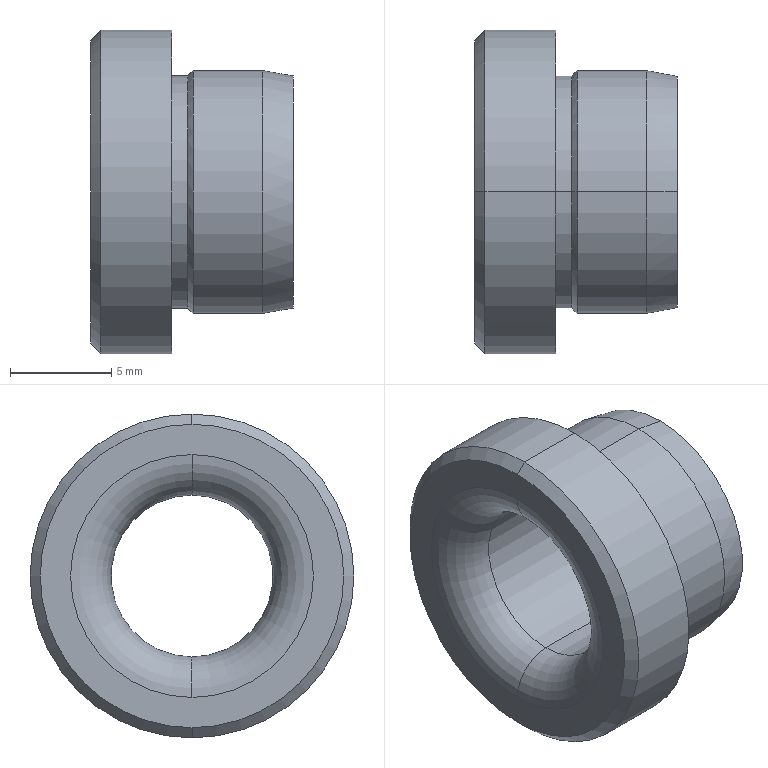Part | NX | features BREP 1 | 1 solid | 23 faces | box 10 x 16 x 16 mm | volume 921.631 mm3 | cylinder 8 | cone 8 | torus 4 | plane 3 | commonest cylinder face diameters 8 x2 11.5 x2 12 x2 16 x2
STEP:
#1=CARTESIAN_POINT('',(0.,0.,6.));
#2=VERTEX_POINT('',#1);
#3=CARTESIAN_POINT('',(0.,0.,-6.));
#4=VERTEX_POINT('',#3);
#5=CARTESIAN_POINT('',(0.,0.,0.));
#6=DIRECTION('',(-1.,0.,0.));
#7=DIRECTION('',(0.,0.,1.));
#8=AXIS2_PLACEMENT_3D('',#5,#6,#7);
#9=CIRCLE('',#8,6.);
#10=EDGE_CURVE('',#2,#4,#9,.T.);
#11=ORIENTED_EDGE('',*,*,#10,.T.);
#12=CARTESIAN_POINT('',(2.,0.,-4.));
#13=VERTEX_POINT('',#12);
#14=CARTESIAN_POINT('',(2.,0.,-6.));
#15=DIRECTION('',(0.,1.,0.));
#16=DIRECTION('',(0.,0.,1.));
#17=AXIS2_PLACEMENT_3D('',#14,#15,#16);
#18=CIRCLE('',#17,2.);
#19=EDGE_CURVE('',#13,#4,#18,.F.);
#20=ORIENTED_EDGE('',*,*,#19,.F.);
#21=CARTESIAN_POINT('',(2.,0.,4.));
#22=VERTEX_POINT('',#21);
#23=CARTESIAN_POINT('',(2.,0.,0.));
#24=DIRECTION('',(-1.,0.,0.));
#25=DIRECTION('',(0.,0.,1.));
#26=AXIS2_PLACEMENT_3D('',#23,#24,#25);
#27=CIRCLE('',#26,4.);
#28=EDGE_CURVE('',#22,#13,#27,.T.);
#29=ORIENTED_EDGE('',*,*,#28,.F.);
#30=CARTESIAN_POINT('',(2.,0.,6.));
#31=DIRECTION('',(0.,-1.,0.));
#32=DIRECTION('',(0.,0.,-1.));
#33=AXIS2_PLACEMENT_3D('',#30,#31,#32);
#34=CIRCLE('',#33,2.);
#35=EDGE_CURVE('',#22,#2,#34,.F.);
#36=ORIENTED_EDGE('',*,*,#35,.T.);
#37=EDGE_LOOP('',(#11,#20,#29,#36));
#38=FACE_BOUND('',#37,.T.);
#39=CARTESIAN_POINT('',(2.,0.,0.));
#40=DIRECTION('',(-1.,0.,0.));
#41=DIRECTION('',(0.,0.,1.));
#42=AXIS2_PLACEMENT_3D('',#39,#40,#41);
#43=TOROIDAL_SURFACE('',#42,6.,2.);
#44=ADVANCED_FACE('',(#38),#43,.T.);
#45=CARTESIAN_POINT('',(10.,0.,-4.));
#46=VERTEX_POINT('',#45);
#47=CARTESIAN_POINT('',(10.,0.,4.));
#48=VERTEX_POINT('',#47);
#49=CARTESIAN_POINT('',(10.,0.,0.));
#50=DIRECTION('',(-1.,0.,0.));
#51=DIRECTION('',(0.,0.,1.));
#52=AXIS2_PLACEMENT_3D('',#49,#50,#51);
#53=CIRCLE('',#52,4.);
#54=EDGE_CURVE('',#46,#48,#53,.T.);
#55=ORIENTED_EDGE('',*,*,#54,.F.);
#56=CARTESIAN_POINT('',(10.,0.,-4.));
#57=DIRECTION('',(-1.,0.,0.));
#58=VECTOR('',#57,1000.);
#59=LINE('',#56,#58);
#60=EDGE_CURVE('',#13,#46,#59,.F.);
#61=ORIENTED_EDGE('',*,*,#60,.F.);
#62=CARTESIAN_POINT('',(2.,0.,0.));
#63=DIRECTION('',(-1.,0.,0.));
#64=DIRECTION('',(0.,0.,1.));
#65=AXIS2_PLACEMENT_3D('',#62,#63,#64);
#66=CIRCLE('',#65,4.);
#67=EDGE_CURVE('',#13,#22,#66,.T.);
#68=ORIENTED_EDGE('',*,*,#67,.T.);
#69=CARTESIAN_POINT('',(10.,0.,4.));
#70=DIRECTION('',(-1.,0.,0.));
#71=VECTOR('',#70,1000.);
#72=LINE('',#69,#71);
#73=EDGE_CURVE('',#22,#48,#72,.F.);
#74=ORIENTED_EDGE('',*,*,#73,.T.);
#75=EDGE_LOOP('',(#55,#61,#68,#74));
#76=FACE_BOUND('',#75,.T.);
#77=CARTESIAN_POINT('',(10.,0.,0.));
#78=DIRECTION('',(-1.,0.,0.));
#79=DIRECTION('',(0.,0.,1.));
#80=AXIS2_PLACEMENT_3D('',#77,#78,#79);
#81=CYLINDRICAL_SURFACE('',#80,4.);
#82=ADVANCED_FACE('',(#76),#81,.F.);
#83=CARTESIAN_POINT('',(8.5,0.,6.));
#84=VERTEX_POINT('',#83);
#85=CARTESIAN_POINT('',(8.5,0.,-6.));
#86=VERTEX_POINT('',#85);
#87=CARTESIAN_POINT('',(8.5,0.,0.));
#88=DIRECTION('',(-1.,0.,0.));
#89=DIRECTION('',(0.,0.,1.));
#90=AXIS2_PLACEMENT_3D('',#87,#88,#89);
#91=CIRCLE('',#90,6.);
#92=EDGE_CURVE('',#84,#86,#91,.T.);
#93=ORIENTED_EDGE('',*,*,#92,.T.);
#94=CARTESIAN_POINT('',(5.05,0.,-6.));
#95=VERTEX_POINT('',#94);
#96=CARTESIAN_POINT('',(10.,0.,-6.));
#97=DIRECTION('',(-1.,0.,0.));
#98=VECTOR('',#97,1000.);
#99=LINE('',#96,#98);
#100=EDGE_CURVE('',#95,#86,#99,.F.);
#101=ORIENTED_EDGE('',*,*,#100,.F.);
#102=CARTESIAN_POINT('',(5.05,0.,6.));
#103=VERTEX_POINT('',#102);
#104=CARTESIAN_POINT('',(5.05,0.,0.));
#105=DIRECTION('',(-1.,0.,0.));
#106=DIRECTION('',(0.,0.,-1.));
#107=AXIS2_PLACEMENT_3D('',#104,#105,#106);
#108=CIRCLE('',#107,6.);
#109=EDGE_CURVE('',#103,#95,#108,.T.);
#110=ORIENTED_EDGE('',*,*,#109,.F.);
#111=CARTESIAN_POINT('',(10.,0.,6.));
#112=DIRECTION('',(-1.,0.,0.));
#113=VECTOR('',#112,1000.);
#114=LINE('',#111,#113);
#115=EDGE_CURVE('',#103,#84,#114,.F.);
#116=ORIENTED_EDGE('',*,*,#115,.T.);
#117=EDGE_LOOP('',(#93,#101,#110,#116));
#118=FACE_BOUND('',#117,.T.);
#119=CARTESIAN_POINT('',(10.,0.,0.));
#120=DIRECTION('',(-1.,0.,0.));
#121=DIRECTION('',(0.,0.,1.));
#122=AXIS2_PLACEMENT_3D('',#119,#120,#121);
#123=CYLINDRICAL_SURFACE('',#122,6.);
#124=ADVANCED_FACE('',(#118),#123,.T.);
#125=CARTESIAN_POINT('',(10.,0.,5.736));
#126=VERTEX_POINT('',#125);
#127=CARTESIAN_POINT('',(10.,0.,-5.736));
#128=VERTEX_POINT('',#127);
#129=CARTESIAN_POINT('',(10.,0.,0.));
#130=DIRECTION('',(-1.,0.,0.));
#131=DIRECTION('',(0.,0.,1.));
#132=AXIS2_PLACEMENT_3D('',#129,#130,#131);
#133=CIRCLE('',#132,5.736);
#134=EDGE_CURVE('',#126,#128,#133,.T.);
#135=ORIENTED_EDGE('',*,*,#134,.T.);
#136=CARTESIAN_POINT('',(10.,0.,-5.736));
#137=DIRECTION('',(-0.9848,0.,-0.1736));
#138=VECTOR('',#137,1000.);
#139=LINE('',#136,#138);
#140=EDGE_CURVE('',#86,#128,#139,.F.);
#141=ORIENTED_EDGE('',*,*,#140,.F.);
#142=ORIENTED_EDGE('',*,*,#92,.F.);
#143=CARTESIAN_POINT('',(10.,0.,5.736));
#144=DIRECTION('',(-0.9848,0.,0.1736));
#145=VECTOR('',#144,1000.);
#146=LINE('',#143,#145);
#147=EDGE_CURVE('',#84,#126,#146,.F.);
#148=ORIENTED_EDGE('',*,*,#147,.T.);
#149=EDGE_LOOP('',(#135,#141,#142,#148));
#150=FACE_BOUND('',#149,.T.);
#151=CARTESIAN_POINT('',(10.,0.,0.));
#152=DIRECTION('',(-1.,0.,0.));
#153=DIRECTION('',(0.,0.,1.));
#154=AXIS2_PLACEMENT_3D('',#151,#152,#153);
#155=CONICAL_SURFACE('',#154,5.736,0.1745);
#156=ADVANCED_FACE('',(#150),#155,.T.);
#157=CARTESIAN_POINT('',(4.8,0.,5.75));
#158=VERTEX_POINT('',#157);
#159=CARTESIAN_POINT('',(4.8,0.,-5.75));
#160=VERTEX_POINT('',#159);
#161=CARTESIAN_POINT('',(4.8,0.,0.));
#162=DIRECTION('',(-1.,0.,0.));
#163=DIRECTION('',(0.,0.,1.));
#164=AXIS2_PLACEMENT_3D('',#161,#162,#163);
#165=CIRCLE('',#164,5.75);
#166=EDGE_CURVE('',#158,#160,#165,.T.);
#167=ORIENTED_EDGE('',*,*,#166,.T.);
#168=CARTESIAN_POINT('',(4.,0.,-5.75));
#169=VERTEX_POINT('',#168);
#170=CARTESIAN_POINT('',(50.,0.,-5.75));
#171=DIRECTION('',(-1.,0.,0.));
#172=VECTOR('',#171,1000.);
#173=LINE('',#170,#172);
#174=EDGE_CURVE('',#169,#160,#173,.F.);
#175=ORIENTED_EDGE('',*,*,#174,.F.);
#176=CARTESIAN_POINT('',(4.,0.,5.75));
#177=VERTEX_POINT('',#176);
#178=CARTESIAN_POINT('',(4.,0.,0.));
#179=DIRECTION('',(-1.,0.,0.));
#180=DIRECTION('',(0.,0.,1.));
#181=AXIS2_PLACEMENT_3D('',#178,#179,#180);
#182=CIRCLE('',#181,5.75);
#183=EDGE_CURVE('',#177,#169,#182,.T.);
#184=ORIENTED_EDGE('',*,*,#183,.F.);
#185=CARTESIAN_POINT('',(50.,0.,5.75));
#186=DIRECTION('',(-1.,0.,0.));
#187=VECTOR('',#186,1000.);
#188=LINE('',#185,#187);
#189=EDGE_CURVE('',#177,#158,#188,.F.);
#190=ORIENTED_EDGE('',*,*,#189,.T.);
#191=EDGE_LOOP('',(#167,#175,#184,#190));
#192=FACE_BOUND('',#191,.T.);
#193=CARTESIAN_POINT('',(50.,0.,0.));
#194=DIRECTION('',(-1.,0.,0.));
#195=DIRECTION('',(0.,0.,1.));
#196=AXIS2_PLACEMENT_3D('',#193,#194,#195);
#197=CYLINDRICAL_SURFACE('',#196,5.75);
#198=ADVANCED_FACE('',(#192),#197,.T.);
#199=CARTESIAN_POINT('',(3.645,0.,-6.335));
#200=VERTEX_POINT('',#199);
#201=CARTESIAN_POINT('',(3.645,0.,6.335));
#202=VERTEX_POINT('',#201);
#203=CARTESIAN_POINT('',(3.645,0.,0.));
#204=DIRECTION('',(-1.,0.,0.));
#205=DIRECTION('',(0.,0.,1.));
#206=AXIS2_PLACEMENT_3D('',#203,#204,#205);
#207=CIRCLE('',#206,6.335);
#208=EDGE_CURVE('',#200,#202,#207,.T.);
#209=ORIENTED_EDGE('',*,*,#208,.F.);
#210=CARTESIAN_POINT('',(4.,0.,-6.15));
#211=DIRECTION('',(0.,1.,0.));
#212=DIRECTION('',(0.,0.,1.));
#213=AXIS2_PLACEMENT_3D('',#210,#211,#212);
#214=CIRCLE('',#213,0.4);
#215=EDGE_CURVE('',#169,#200,#214,.F.);
#216=ORIENTED_EDGE('',*,*,#215,.F.);
#217=CARTESIAN_POINT('',(4.,0.,0.));
#218=DIRECTION('',(-1.,0.,0.));
#219=DIRECTION('',(0.,0.,1.));
#220=AXIS2_PLACEMENT_3D('',#217,#218,#219);
#221=CIRCLE('',#220,5.75);
#222=EDGE_CURVE('',#169,#177,#221,.T.);
#223=ORIENTED_EDGE('',*,*,#222,.T.);
#224=CARTESIAN_POINT('',(4.,0.,6.15));
#225=DIRECTION('',(0.,-1.,0.));
#226=DIRECTION('',(0.,0.,-1.));
#227=AXIS2_PLACEMENT_3D('',#224,#225,#226);
#228=CIRCLE('',#227,0.4);
#229=EDGE_CURVE('',#177,#202,#228,.F.);
#230=ORIENTED_EDGE('',*,*,#229,.T.);
#231=EDGE_LOOP('',(#209,#216,#223,#230));
#232=FACE_BOUND('',#231,.T.);
#233=CARTESIAN_POINT('',(4.,0.,0.));
#234=DIRECTION('',(-1.,0.,0.));
#235=DIRECTION('',(0.,0.,1.));
#236=AXIS2_PLACEMENT_3D('',#233,#234,#235);
#237=TOROIDAL_SURFACE('',#236,6.15,0.4);
#238=ADVANCED_FACE('',(#232),#237,.F.);
#239=ORIENTED_EDGE('',*,*,#166,.F.);
#240=CARTESIAN_POINT('',(4.8,0.,5.75));
#241=DIRECTION('',(0.7071,0.,0.7071));
#242=VECTOR('',#241,1000.);
#243=LINE('',#240,#242);
#244=EDGE_CURVE('',#158,#103,#243,.T.);
#245=ORIENTED_EDGE('',*,*,#244,.T.);
#246=ORIENTED_EDGE('',*,*,#109,.T.);
#247=CARTESIAN_POINT('',(4.8,0.,-5.75));
#248=DIRECTION('',(0.7071,0.,-0.7071));
#249=VECTOR('',#248,1000.);
#250=LINE('',#247,#249);
#251=EDGE_CURVE('',#160,#95,#250,.T.);
#252=ORIENTED_EDGE('',*,*,#251,.F.);
#253=EDGE_LOOP('',(#239,#245,#246,#252));
#254=FACE_BOUND('',#253,.T.);
#255=CARTESIAN_POINT('',(4.8,0.,0.));
#256=DIRECTION('',(1.,0.,0.));
#257=DIRECTION('',(0.,0.,-1.));
#258=AXIS2_PLACEMENT_3D('',#255,#256,#257);
#259=CONICAL_SURFACE('',#258,5.75,0.7854);
#260=ADVANCED_FACE('',(#254),#259,.T.);
#261=ORIENTED_EDGE('',*,*,#208,.T.);
#262=CARTESIAN_POINT('',(4.,0.,7.016));
#263=VERTEX_POINT('',#262);
#264=CARTESIAN_POINT('',(4.122,0.,7.25));
#265=DIRECTION('',(0.4617,0.,0.887));
#266=VECTOR('',#265,1000.);
#267=LINE('',#264,#266);
#268=EDGE_CURVE('',#202,#263,#267,.T.);
#269=ORIENTED_EDGE('',*,*,#268,.T.);
#270=CARTESIAN_POINT('',(4.,0.,-7.016));
#271=VERTEX_POINT('',#270);
#272=CARTESIAN_POINT('',(4.,0.,0.));
#273=DIRECTION('',(1.,0.,0.));
#274=DIRECTION('',(0.,0.,1.));
#275=AXIS2_PLACEMENT_3D('',#272,#273,#274);
#276=CIRCLE('',#275,7.016);
#277=EDGE_CURVE('',#263,#271,#276,.T.);
#278=ORIENTED_EDGE('',*,*,#277,.T.);
#279=CARTESIAN_POINT('',(4.122,0.,-7.25));
#280=DIRECTION('',(0.4617,0.,-0.887));
#281=VECTOR('',#280,1000.);
#282=LINE('',#279,#281);
#283=EDGE_CURVE('',#200,#271,#282,.T.);
#284=ORIENTED_EDGE('',*,*,#283,.F.);
#285=EDGE_LOOP('',(#261,#269,#278,#284));
#286=FACE_BOUND('',#285,.T.);
#287=CARTESIAN_POINT('',(4.122,0.,0.));
#288=DIRECTION('',(1.,0.,0.));
#289=DIRECTION('',(0.,0.,-1.));
#290=AXIS2_PLACEMENT_3D('',#287,#288,#289);
#291=CONICAL_SURFACE('',#290,7.25,1.091);
#292=ADVANCED_FACE('',(#286),#291,.F.);
#293=CARTESIAN_POINT('',(4.,0.,8.));
#294=VERTEX_POINT('',#293);
#295=CARTESIAN_POINT('',(4.,0.,-8.));
#296=VERTEX_POINT('',#295);
#297=CARTESIAN_POINT('',(4.,0.,0.));
#298=DIRECTION('',(-1.,0.,0.));
#299=DIRECTION('',(0.,0.,1.));
#300=AXIS2_PLACEMENT_3D('',#297,#298,#299);
#301=CIRCLE('',#300,8.);
#302=EDGE_CURVE('',#294,#296,#301,.T.);
#303=ORIENTED_EDGE('',*,*,#302,.T.);
#304=CARTESIAN_POINT('',(0.5,0.,-8.));
#305=VERTEX_POINT('',#304);
#306=CARTESIAN_POINT('',(10.,0.,-8.));
#307=DIRECTION('',(-1.,0.,0.));
#308=VECTOR('',#307,1000.);
#309=LINE('',#306,#308);
#310=EDGE_CURVE('',#305,#296,#309,.F.);
#311=ORIENTED_EDGE('',*,*,#310,.F.);
#312=CARTESIAN_POINT('',(0.5,0.,8.));
#313=VERTEX_POINT('',#312);
#314=CARTESIAN_POINT('',(0.5,0.,0.));
#315=DIRECTION('',(-1.,0.,0.));
#316=DIRECTION('',(0.,0.,1.));
#317=AXIS2_PLACEMENT_3D('',#314,#315,#316);
#318=CIRCLE('',#317,8.);
#319=EDGE_CURVE('',#313,#305,#318,.T.);
#320=ORIENTED_EDGE('',*,*,#319,.F.);
#321=CARTESIAN_POINT('',(10.,0.,8.));
#322=DIRECTION('',(-1.,0.,0.));
#323=VECTOR('',#322,1000.);
#324=LINE('',#321,#323);
#325=EDGE_CURVE('',#313,#294,#324,.F.);
#326=ORIENTED_EDGE('',*,*,#325,.T.);
#327=EDGE_LOOP('',(#303,#311,#320,#326));
#328=FACE_BOUND('',#327,.T.);
#329=CARTESIAN_POINT('',(10.,0.,0.));
#330=DIRECTION('',(-1.,0.,0.));
#331=DIRECTION('',(0.,0.,1.));
#332=AXIS2_PLACEMENT_3D('',#329,#330,#331);
#333=CYLINDRICAL_SURFACE('',#332,8.);
#334=ADVANCED_FACE('',(#328),#333,.T.);
#335=CARTESIAN_POINT('',(0.,0.,7.5));
#336=VERTEX_POINT('',#335);
#337=CARTESIAN_POINT('',(0.,0.,-7.5));
#338=VERTEX_POINT('',#337);
#339=CARTESIAN_POINT('',(0.,0.,0.));
#340=DIRECTION('',(-1.,0.,0.));
#341=DIRECTION('',(0.,0.,1.));
#342=AXIS2_PLACEMENT_3D('',#339,#340,#341);
#343=CIRCLE('',#342,7.5);
#344=EDGE_CURVE('',#336,#338,#343,.T.);
#345=ORIENTED_EDGE('',*,*,#344,.F.);
#346=CARTESIAN_POINT('',(0.5,0.,8.));
#347=DIRECTION('',(0.7071,0.,0.7071));
#348=VECTOR('',#347,1000.);
#349=LINE('',#346,#348);
#350=EDGE_CURVE('',#336,#313,#349,.T.);
#351=ORIENTED_EDGE('',*,*,#350,.T.);
#352=ORIENTED_EDGE('',*,*,#319,.T.);
#353=CARTESIAN_POINT('',(0.5,0.,-8.));
#354=DIRECTION('',(0.7071,0.,-0.7071));
#355=VECTOR('',#354,1000.);
#356=LINE('',#353,#355);
#357=EDGE_CURVE('',#338,#305,#356,.T.);
#358=ORIENTED_EDGE('',*,*,#357,.F.);
#359=EDGE_LOOP('',(#345,#351,#352,#358));
#360=FACE_BOUND('',#359,.T.);
#361=CARTESIAN_POINT('',(0.5,0.,0.));
#362=DIRECTION('',(1.,0.,0.));
#363=DIRECTION('',(0.,0.,-1.));
#364=AXIS2_PLACEMENT_3D('',#361,#362,#363);
#365=CONICAL_SURFACE('',#364,8.,0.7854);
#366=ADVANCED_FACE('',(#360),#365,.T.);
#367=CARTESIAN_POINT('',(0.,0.,0.));
#368=DIRECTION('',(-1.,0.,0.));
#369=DIRECTION('',(0.,0.,1.));
#370=AXIS2_PLACEMENT_3D('',#367,#368,#369);
#371=CIRCLE('',#370,7.5);
#372=EDGE_CURVE('',#338,#336,#371,.T.);
#373=ORIENTED_EDGE('',*,*,#372,.T.);
#374=ORIENTED_EDGE('',*,*,#344,.T.);
#375=EDGE_LOOP('',(#373,#374));
#376=FACE_BOUND('',#375,.T.);
#377=ORIENTED_EDGE('',*,*,#10,.F.);
#378=CARTESIAN_POINT('',(0.,0.,0.));
#379=DIRECTION('',(-1.,0.,0.));
#380=DIRECTION('',(0.,0.,1.));
#381=AXIS2_PLACEMENT_3D('',#378,#379,#380);
#382=CIRCLE('',#381,6.);
#383=EDGE_CURVE('',#4,#2,#382,.T.);
#384=ORIENTED_EDGE('',*,*,#383,.F.);
#385=EDGE_LOOP('',(#377,#384));
#386=FACE_BOUND('',#385,.T.);
#387=CARTESIAN_POINT('',(0.,0.,0.));
#388=DIRECTION('',(1.,0.,0.));
#389=DIRECTION('',(0.,1.,0.));
#390=AXIS2_PLACEMENT_3D('',#387,#388,#389);
#391=PLANE('',#390);
#392=ADVANCED_FACE('',(#376,#386),#391,.F.);
#393=ORIENTED_EDGE('',*,*,#134,.F.);
#394=CARTESIAN_POINT('',(10.,0.,0.));
#395=DIRECTION('',(-1.,0.,0.));
#396=DIRECTION('',(0.,0.,1.));
#397=AXIS2_PLACEMENT_3D('',#394,#395,#396);
#398=CIRCLE('',#397,5.736);
#399=EDGE_CURVE('',#128,#126,#398,.T.);
#400=ORIENTED_EDGE('',*,*,#399,.F.);
#401=EDGE_LOOP('',(#393,#400));
#402=FACE_BOUND('',#401,.T.);
#403=CARTESIAN_POINT('',(10.,0.,0.));
#404=DIRECTION('',(-1.,0.,0.));
#405=DIRECTION('',(0.,0.,1.));
#406=AXIS2_PLACEMENT_3D('',#403,#404,#405);
#407=CIRCLE('',#406,4.);
#408=EDGE_CURVE('',#48,#46,#407,.T.);
#409=ORIENTED_EDGE('',*,*,#408,.T.);
#410=ORIENTED_EDGE('',*,*,#54,.T.);
#411=EDGE_LOOP('',(#409,#410));
#412=FACE_BOUND('',#411,.T.);
#413=CARTESIAN_POINT('',(10.,5.736,0.));
#414=DIRECTION('',(-1.,0.,0.));
#415=DIRECTION('',(0.,0.,1.));
#416=AXIS2_PLACEMENT_3D('',#413,#414,#415);
#417=PLANE('',#416);
#418=ADVANCED_FACE('',(#402,#412),#417,.F.);
#419=ORIENTED_EDGE('',*,*,#302,.F.);
#420=CARTESIAN_POINT('',(4.,0.,0.));
#421=DIRECTION('',(-1.,0.,0.));
#422=DIRECTION('',(0.,0.,1.));
#423=AXIS2_PLACEMENT_3D('',#420,#421,#422);
#424=CIRCLE('',#423,8.);
#425=EDGE_CURVE('',#296,#294,#424,.T.);
#426=ORIENTED_EDGE('',*,*,#425,.F.);
#427=EDGE_LOOP('',(#419,#426));
#428=FACE_BOUND('',#427,.T.);
#429=CARTESIAN_POINT('',(4.,0.,0.));
#430=DIRECTION('',(1.,0.,0.));
#431=DIRECTION('',(0.,0.,1.));
#432=AXIS2_PLACEMENT_3D('',#429,#430,#431);
#433=CIRCLE('',#432,7.016);
#434=EDGE_CURVE('',#271,#263,#433,.T.);
#435=ORIENTED_EDGE('',*,*,#434,.F.);
#436=ORIENTED_EDGE('',*,*,#277,.F.);
#437=EDGE_LOOP('',(#435,#436));
#438=FACE_BOUND('',#437,.T.);
#439=CARTESIAN_POINT('',(4.,8.,0.));
#440=DIRECTION('',(-1.,0.,0.));
#441=DIRECTION('',(0.,0.,1.));
#442=AXIS2_PLACEMENT_3D('',#439,#440,#441);
#443=PLANE('',#442);
#444=ADVANCED_FACE('',(#428,#438),#443,.F.);
#445=ORIENTED_EDGE('',*,*,#350,.F.);
#446=ORIENTED_EDGE('',*,*,#372,.F.);
#447=ORIENTED_EDGE('',*,*,#357,.T.);
#448=CARTESIAN_POINT('',(0.5,0.,0.));
#449=DIRECTION('',(-1.,0.,0.));
#450=DIRECTION('',(0.,0.,1.));
#451=AXIS2_PLACEMENT_3D('',#448,#449,#450);
#452=CIRCLE('',#451,8.);
#453=EDGE_CURVE('',#305,#313,#452,.T.);
#454=ORIENTED_EDGE('',*,*,#453,.T.);
#455=EDGE_LOOP('',(#445,#446,#447,#454));
#456=FACE_BOUND('',#455,.T.);
#457=CARTESIAN_POINT('',(0.5,0.,0.));
#458=DIRECTION('',(1.,0.,0.));
#459=DIRECTION('',(0.,0.,-1.));
#460=AXIS2_PLACEMENT_3D('',#457,#458,#459);
#461=CONICAL_SURFACE('',#460,8.,0.7854);
#462=ADVANCED_FACE('',(#456),#461,.T.);
#463=ORIENTED_EDGE('',*,*,#310,.T.);
#464=ORIENTED_EDGE('',*,*,#425,.T.);
#465=ORIENTED_EDGE('',*,*,#325,.F.);
#466=ORIENTED_EDGE('',*,*,#453,.F.);
#467=EDGE_LOOP('',(#463,#464,#465,#466));
#468=FACE_BOUND('',#467,.T.);
#469=CARTESIAN_POINT('',(10.,0.,0.));
#470=DIRECTION('',(-1.,0.,0.));
#471=DIRECTION('',(0.,0.,1.));
#472=AXIS2_PLACEMENT_3D('',#469,#470,#471);
#473=CYLINDRICAL_SURFACE('',#472,8.);
#474=ADVANCED_FACE('',(#468),#473,.T.);
#475=ORIENTED_EDGE('',*,*,#268,.F.);
#476=CARTESIAN_POINT('',(3.645,0.,0.));
#477=DIRECTION('',(-1.,0.,0.));
#478=DIRECTION('',(0.,0.,1.));
#479=AXIS2_PLACEMENT_3D('',#476,#477,#478);
#480=CIRCLE('',#479,6.335);
#481=EDGE_CURVE('',#202,#200,#480,.T.);
#482=ORIENTED_EDGE('',*,*,#481,.T.);
#483=ORIENTED_EDGE('',*,*,#283,.T.);
#484=ORIENTED_EDGE('',*,*,#434,.T.);
#485=EDGE_LOOP('',(#475,#482,#483,#484));
#486=FACE_BOUND('',#485,.T.);
#487=CARTESIAN_POINT('',(4.122,0.,0.));
#488=DIRECTION('',(1.,0.,0.));
#489=DIRECTION('',(0.,0.,-1.));
#490=AXIS2_PLACEMENT_3D('',#487,#488,#489);
#491=CONICAL_SURFACE('',#490,7.25,1.091);
#492=ADVANCED_FACE('',(#486),#491,.F.);
#493=ORIENTED_EDGE('',*,*,#244,.F.);
#494=CARTESIAN_POINT('',(4.8,0.,0.));
#495=DIRECTION('',(-1.,0.,0.));
#496=DIRECTION('',(0.,0.,1.));
#497=AXIS2_PLACEMENT_3D('',#494,#495,#496);
#498=CIRCLE('',#497,5.75);
#499=EDGE_CURVE('',#160,#158,#498,.T.);
#500=ORIENTED_EDGE('',*,*,#499,.F.);
#501=ORIENTED_EDGE('',*,*,#251,.T.);
#502=CARTESIAN_POINT('',(5.05,0.,0.));
#503=DIRECTION('',(-1.,0.,0.));
#504=DIRECTION('',(0.,0.,-1.));
#505=AXIS2_PLACEMENT_3D('',#502,#503,#504);
#506=CIRCLE('',#505,6.);
#507=EDGE_CURVE('',#95,#103,#506,.T.);
#508=ORIENTED_EDGE('',*,*,#507,.T.);
#509=EDGE_LOOP('',(#493,#500,#501,#508));
#510=FACE_BOUND('',#509,.T.);
#511=CARTESIAN_POINT('',(4.8,0.,0.));
#512=DIRECTION('',(1.,0.,0.));
#513=DIRECTION('',(0.,0.,-1.));
#514=AXIS2_PLACEMENT_3D('',#511,#512,#513);
#515=CONICAL_SURFACE('',#514,5.75,0.7854);
#516=ADVANCED_FACE('',(#510),#515,.T.);
#517=ORIENTED_EDGE('',*,*,#215,.T.);
#518=ORIENTED_EDGE('',*,*,#481,.F.);
#519=ORIENTED_EDGE('',*,*,#229,.F.);
#520=ORIENTED_EDGE('',*,*,#183,.T.);
#521=EDGE_LOOP('',(#517,#518,#519,#520));
#522=FACE_BOUND('',#521,.T.);
#523=CARTESIAN_POINT('',(4.,0.,0.));
#524=DIRECTION('',(-1.,0.,0.));
#525=DIRECTION('',(0.,0.,1.));
#526=AXIS2_PLACEMENT_3D('',#523,#524,#525);
#527=TOROIDAL_SURFACE('',#526,6.15,0.4);
#528=ADVANCED_FACE('',(#522),#527,.F.);
#529=ORIENTED_EDGE('',*,*,#174,.T.);
#530=ORIENTED_EDGE('',*,*,#499,.T.);
#531=ORIENTED_EDGE('',*,*,#189,.F.);
#532=ORIENTED_EDGE('',*,*,#222,.F.);
#533=EDGE_LOOP('',(#529,#530,#531,#532));
#534=FACE_BOUND('',#533,.T.);
#535=CARTESIAN_POINT('',(50.,0.,0.));
#536=DIRECTION('',(-1.,0.,0.));
#537=DIRECTION('',(0.,0.,1.));
#538=AXIS2_PLACEMENT_3D('',#535,#536,#537);
#539=CYLINDRICAL_SURFACE('',#538,5.75);
#540=ADVANCED_FACE('',(#534),#539,.T.);
#541=ORIENTED_EDGE('',*,*,#140,.T.);
#542=ORIENTED_EDGE('',*,*,#399,.T.);
#543=ORIENTED_EDGE('',*,*,#147,.F.);
#544=CARTESIAN_POINT('',(8.5,0.,0.));
#545=DIRECTION('',(-1.,0.,0.));
#546=DIRECTION('',(0.,0.,1.));
#547=AXIS2_PLACEMENT_3D('',#544,#545,#546);
#548=CIRCLE('',#547,6.);
#549=EDGE_CURVE('',#86,#84,#548,.T.);
#550=ORIENTED_EDGE('',*,*,#549,.F.);
#551=EDGE_LOOP('',(#541,#542,#543,#550));
#552=FACE_BOUND('',#551,.T.);
#553=CARTESIAN_POINT('',(10.,0.,0.));
#554=DIRECTION('',(-1.,0.,0.));
#555=DIRECTION('',(0.,0.,1.));
#556=AXIS2_PLACEMENT_3D('',#553,#554,#555);
#557=CONICAL_SURFACE('',#556,5.736,0.1745);
#558=ADVANCED_FACE('',(#552),#557,.T.);
#559=ORIENTED_EDGE('',*,*,#100,.T.);
#560=ORIENTED_EDGE('',*,*,#549,.T.);
#561=ORIENTED_EDGE('',*,*,#115,.F.);
#562=ORIENTED_EDGE('',*,*,#507,.F.);
#563=EDGE_LOOP('',(#559,#560,#561,#562));
#564=FACE_BOUND('',#563,.T.);
#565=CARTESIAN_POINT('',(10.,0.,0.));
#566=DIRECTION('',(-1.,0.,0.));
#567=DIRECTION('',(0.,0.,1.));
#568=AXIS2_PLACEMENT_3D('',#565,#566,#567);
#569=CYLINDRICAL_SURFACE('',#568,6.);
#570=ADVANCED_FACE('',(#564),#569,.T.);
#571=ORIENTED_EDGE('',*,*,#60,.T.);
#572=ORIENTED_EDGE('',*,*,#408,.F.);
#573=ORIENTED_EDGE('',*,*,#73,.F.);
#574=ORIENTED_EDGE('',*,*,#28,.T.);
#575=EDGE_LOOP('',(#571,#572,#573,#574));
#576=FACE_BOUND('',#575,.T.);
#577=CARTESIAN_POINT('',(10.,0.,0.));
#578=DIRECTION('',(-1.,0.,0.));
#579=DIRECTION('',(0.,0.,1.));
#580=AXIS2_PLACEMENT_3D('',#577,#578,#579);
#581=CYLINDRICAL_SURFACE('',#580,4.);
#582=ADVANCED_FACE('',(#576),#581,.F.);
#583=ORIENTED_EDGE('',*,*,#19,.T.);
#584=ORIENTED_EDGE('',*,*,#383,.T.);
#585=ORIENTED_EDGE('',*,*,#35,.F.);
#586=ORIENTED_EDGE('',*,*,#67,.F.);
#587=EDGE_LOOP('',(#583,#584,#585,#586));
#588=FACE_BOUND('',#587,.T.);
#589=CARTESIAN_POINT('',(2.,0.,0.));
#590=DIRECTION('',(-1.,0.,0.));
#591=DIRECTION('',(0.,0.,1.));
#592=AXIS2_PLACEMENT_3D('',#589,#590,#591);
#593=TOROIDAL_SURFACE('',#592,6.,2.);
#594=ADVANCED_FACE('',(#588),#593,.T.);
#595=CLOSED_SHELL('',(#44,#82,#124,#156,#198,#238,#260,#292,#334,#366,#392,#418,#444,#462,#474,#492,#516,#528,#540,#558,#570,#582,#594));
#596=MANIFOLD_SOLID_BREP('',#595);
#597=(LENGTH_UNIT()NAMED_UNIT(*)SI_UNIT(.MILLI.,.METRE.));
#598=UNCERTAINTY_MEASURE_WITH_UNIT(LENGTH_MEASURE(0.00001),#597,'','');
#599=(NAMED_UNIT(*)PLANE_ANGLE_UNIT()SI_UNIT($,.RADIAN.));
#600=(NAMED_UNIT(*)SI_UNIT($,.STERADIAN.)SOLID_ANGLE_UNIT());
#601=(GEOMETRIC_REPRESENTATION_CONTEXT(3)GLOBAL_UNCERTAINTY_ASSIGNED_CONTEXT((#598))GLOBAL_UNIT_ASSIGNED_CONTEXT((#597,#599,#600))REPRESENTATION_CONTEXT('',''));
#602=ADVANCED_BREP_SHAPE_REPRESENTATION('',(#596),#601);